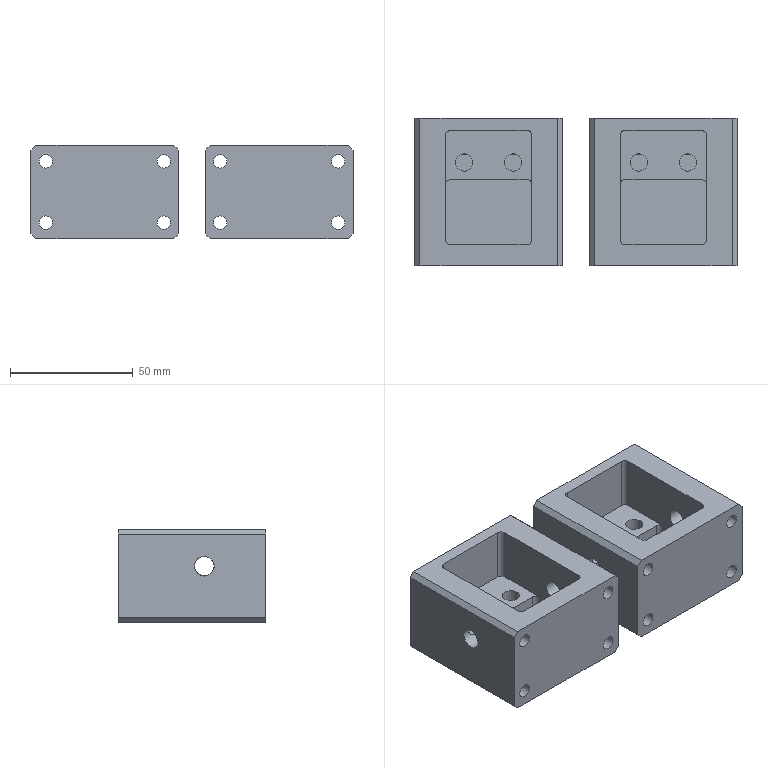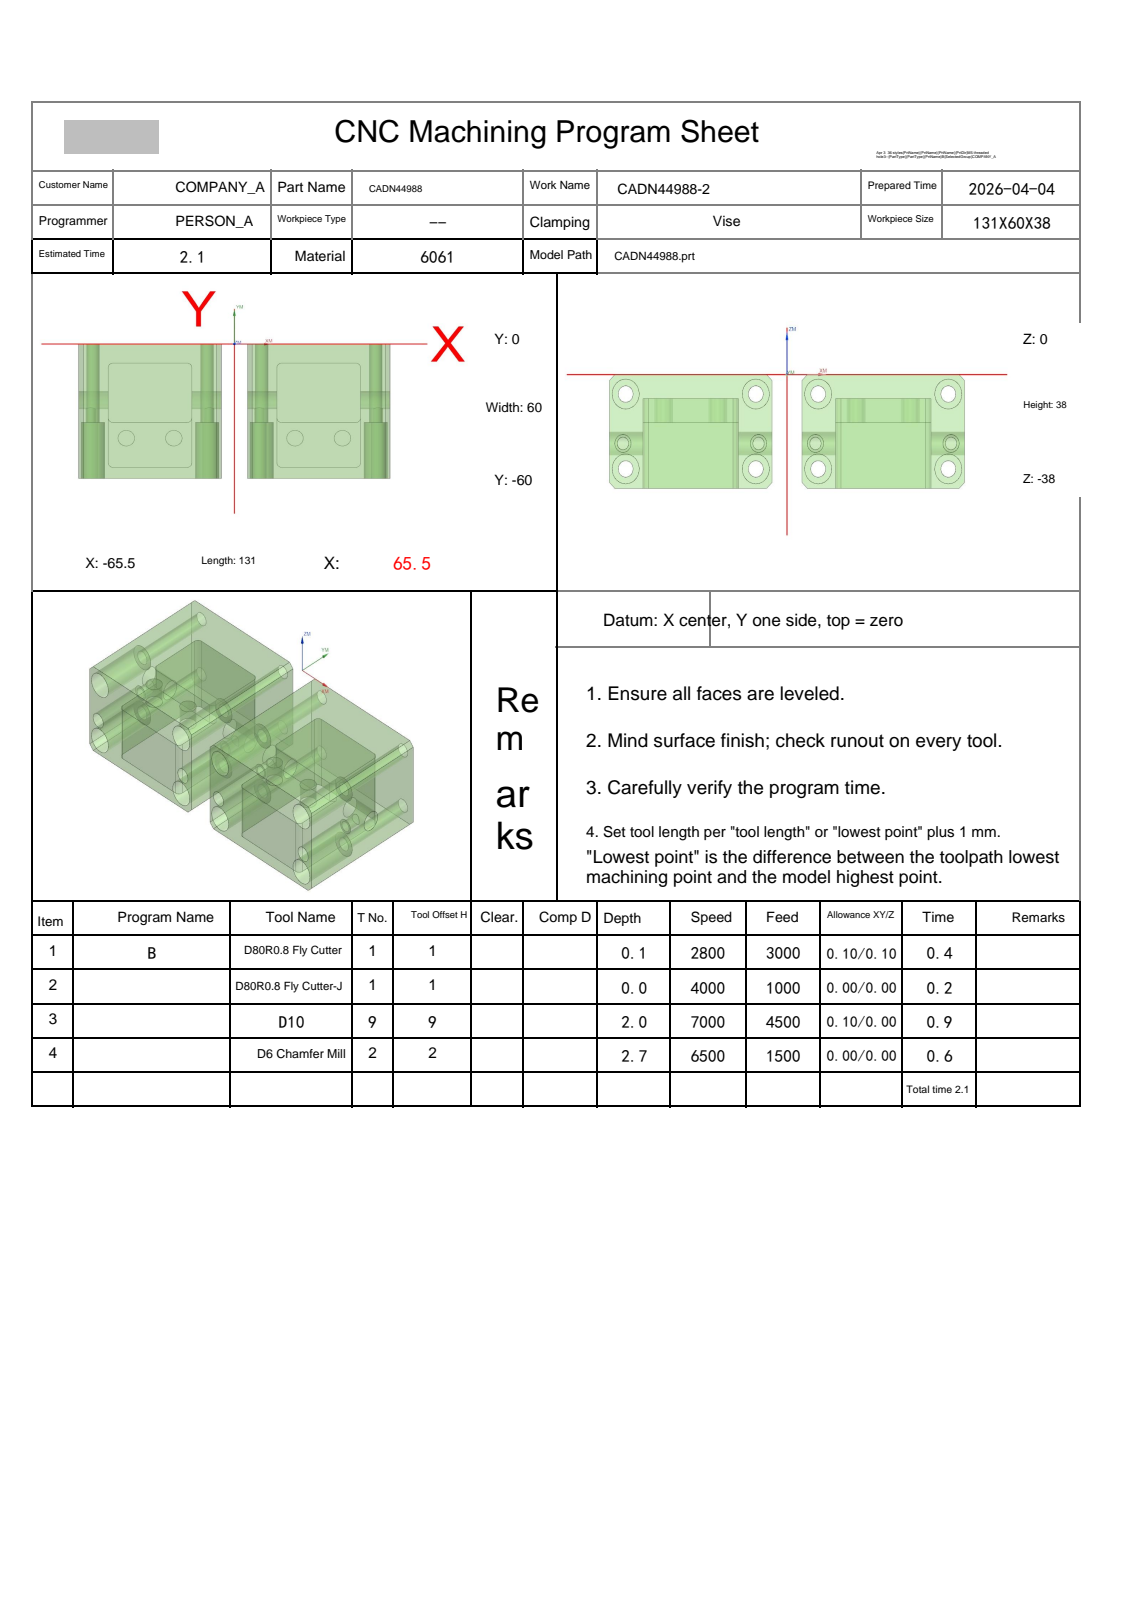NC program | NX | posted by the shop | part box 131 x 60 x 38 mm
Whole program:
%
O0001
(Machine time: 2.90 MIN)
(===Total Tool:3===)
(T1=D80R0.8 Fly Cutter D=80.  R=0.8  D-  H01 Z=0.    )
(T9=D10     D=10.  R=0.   D-  H09 Z=-2.   )
(T2=D6 Chamfer Mill   D=6.   R=0.   D-  H02 Z=-2.7  )
G80 G90 G17 G49 G40
G91 G28 Z0
M01
N1 T01 M06
(D80R0.8 Fly Cutter  D=80. R=0.8 H=01 ce=0.10 di=0.10)
G00 G90 G54 X117.597 Y-30. M03 S2800
G43 H01 Z50.
M08
Z3.525
G01 Z1.525 F3000.
X105.597
X-105.597
X-117.597
Z3.525
G00 X117.597
Z3.05
G01 Z1.05
X105.597
X-105.597
X-117.597
Z3.05
G00 X117.597
Z2.575
G01 Z.575
X105.597
X-105.597
X-117.597
Z2.575
G00 X117.597
Z2.1
G01 Z.1
X105.597
X-105.597
X-117.597
Z2.1
G00 Z50.
G91 G28 Z0.0
M05
M09
G91 G28 Z0.0
M01
N2 T01 M06
(D80R0.8 Fly Cutter-J  D=80. R=0.8 H=01 ce=0.00 di=0.00)
G00 G90 G54 X117.499 Y-30. M03 S4000
G43 H01 Z50.
M08
Z2.
G01 Z0.0 F1000.
X105.499
X-105.499
X-117.499
Z2.
G00 Z50.
G91 G28 Z0.0
M05
M09
G91 G28 Z0.0
M01
N3 T09 M06
(D10  D=10. R=0. H=09 ce=0.10 di=0.00)
G00 G90 G54 X68.442 Y9.956 M03 S7000
G43 H09 Z11.8
M08
Z.359
G01 Z-.141 F4500.
X68.739 Y1.072
X68.741 Y1.014
Y-61.014
X68.739 Y-61.072
X68.812 Z-.212
X68.881 Z-.283
X68.883 Y-61.014
Y1.014
X68.881 Y1.072
X68.954 Z-.354
X69.022 Z-.424
X69.024 Y1.014
Y-61.014
X69.022 Y-61.072
X69.095 Z-.495
X69.164 Z-.566
X69.166 Y-61.014
Y1.014
X69.164 Y1.073
X69.236 Z-.636
X69.305 Z-.707
X69.307 Y1.014
Y-61.014
X69.305 Y-61.073
X69.378 Z-.778
X69.447 Z-.849
X69.449 Y-61.014
Y1.014
X69.447 Y1.073
X69.519 Z-.919
X69.588 Z-.99
X69.59 Y1.014
Y-61.014
X69.588 Y-61.073
X69.661 Z-1.061
X69.729 Z-1.131
X69.731 Y-61.014
Y1.014
X69.729 Y1.073
X69.802 Z-1.202
X69.871 Z-1.273
X69.873 Y1.014
Y-61.014
X69.871 Y-61.073
X69.944 Z-1.344
X70.012 Z-1.414
X70.014 Y-61.014
Y1.014
X70.012 Y1.073
X70.085 Y1.072 Z-1.485
X70.154 Z-1.556
X70.156 Y1.014
Y-61.014
X70.154 Y-61.072
X70.211 Z-1.611
X70.265 Z-1.667
X70.267 Y-61.014
Y1.014
X70.265 Y1.072
X70.322 Z-1.722
X70.376 Z-1.778
X70.378 Y1.014
Y-61.014
X70.376 Y-61.072
X70.433 Z-1.833
X70.487 Z-1.889
X70.489 Y-61.014
Y1.014
X70.487 Y1.072
X70.544 Z-1.944
X70.598 Z-2.
Y-61.072
G00 Z11.8
X2.558 Y-69.955
Z.359
G01 Z-.141
X2.261 Y-61.072
X2.259 Y-61.014
Y1.014
X2.261 Y1.072
X2.188 Z-.212
X2.119 Z-.283
X2.117 Y1.014
Y-61.014
X2.119 Y-61.072
X2.046 Z-.354
X1.978 Z-.424
X1.976 Y-61.014
Y1.014
X1.978 Y1.072
X1.905 Y1.073 Z-.495
X1.836 Z-.566
X1.834 Y1.014
Y-61.014
X1.836 Y-61.073
X1.764 Z-.636
X1.695 Z-.707
X1.693 Y-61.014
Y1.014
X1.695 Y1.073
X1.622 Z-.778
X1.553 Z-.849
X1.551 Y1.014
Y-61.014
X1.553 Y-61.073
X1.481 Z-.919
X1.412 Z-.99
X1.41 Y-61.014
Y1.014
X1.412 Y1.073
X1.339 Z-1.061
X1.271 Z-1.131
X1.269 Y1.014
Y-61.014
X1.271 Y-61.073
X1.198 Z-1.202
X1.129 Z-1.273
X1.127 Y-61.014
Y1.014
X1.129 Y1.073
X1.056 Z-1.344
X.988 Z-1.414
X.986 Y1.014
Y-61.014
X.988 Y-61.073
X.915 Z-1.485
X.846 Y-61.072 Z-1.556
X.844 Y-61.014
Y1.014
X.846 Y1.072
X.789 Z-1.611
X.735 Z-1.667
X.733 Y1.014
Y-61.014
X.735 Y-61.072
X.678 Z-1.722
X.624 Z-1.778
X.622 Y-61.014
Y1.014
X.624 Y1.072
X.567 Z-1.833
X.513 Z-1.889
X.511 Y1.014
Y-61.014
X.513 Y-61.072
X.456 Z-1.944
X.402 Z-2.
Y1.072
G00 Z11.8
X-2.558 Y9.955
Z.359
G01 Z-.141
X-2.261 Y1.072
X-2.259 Y1.014
Y-61.014
X-2.261 Y-61.072
X-2.188 Z-.212
X-2.119 Z-.283
X-2.117 Y-61.014
Y1.014
X-2.119 Y1.072
X-2.046 Z-.354
X-1.978 Z-.424
X-1.976 Y1.014
Y-61.014
X-1.978 Y-61.072
X-1.905 Z-.495
X-1.836 Y-61.073 Z-.566
X-1.834 Y-61.014
Y1.014
X-1.836 Y1.073
X-1.764 Z-.636
X-1.695 Z-.707
X-1.693 Y1.014
Y-61.014
X-1.695 Y-61.073
X-1.622 Z-.778
X-1.553 Z-.849
X-1.551 Y-61.014
Y1.014
X-1.553 Y1.073
X-1.481 Z-.919
X-1.412 Z-.99
X-1.41 Y1.014
Y-61.014
X-1.412 Y-61.073
X-1.339 Z-1.061
X-1.271 Z-1.131
X-1.269 Y-61.014
Y1.014
X-1.271 Y1.073
X-1.198 Z-1.202
X-1.129 Z-1.273
X-1.127 Y1.014
Y-61.014
X-1.129 Y-61.073
X-1.056 Z-1.344
X-.988 Z-1.414
X-.986 Y-61.014
Y1.014
X-.988 Y1.073
X-.915 Y1.072 Z-1.485
X-.846 Z-1.556
X-.844 Y1.014
Y-61.014
X-.846 Y-61.072
X-.789 Z-1.611
X-.735 Z-1.667
X-.733 Y-61.014
Y1.014
X-.735 Y1.072
X-.678 Z-1.722
X-.624 Z-1.778
X-.622 Y1.014
Y-61.014
X-.624 Y-61.072
X-.567 Z-1.833
X-.513 Z-1.889
X-.511 Y-61.014
Y1.014
X-.513 Y1.072
X-.456 Z-1.944
X-.402 Z-2.
Y-61.072
G00 Z11.8
X-68.442 Y-69.956
Z.359
G01 Z-.141
X-68.739 Y-61.072
X-68.741 Y-61.014
Y1.014
X-68.739 Y1.072
X-68.812 Z-.212
X-68.881 Z-.283
X-68.883 Y1.014
Y-61.014
X-68.881 Y-61.072
X-68.954 Z-.354
X-69.022 Z-.424
X-69.024 Y-61.014
Y1.014
X-69.022 Y1.072
X-69.095 Z-.495
X-69.164 Y1.073 Z-.566
X-69.166 Y1.014
Y-61.014
X-69.164 Y-61.072
X-69.236 Y-61.073 Z-.636
X-69.305 Z-.707
X-69.307 Y-61.014
Y1.014
X-69.305 Y1.073
X-69.378 Z-.778
X-69.447 Z-.849
X-69.449 Y1.014
Y-61.014
X-69.447 Y-61.073
X-69.519 Z-.919
X-69.588 Z-.99
X-69.59 Y-61.014
Y1.014
X-69.588 Y1.073
X-69.661 Z-1.061
X-69.729 Z-1.131
X-69.731 Y1.014
Y-61.014
X-69.729 Y-61.073
X-69.802 Z-1.202
X-69.871 Z-1.273
X-69.873 Y-61.014
Y1.014
X-69.871 Y1.073
X-69.944 Z-1.344
X-70.012 Z-1.414
X-70.014 Y1.014
Y-61.014
X-70.012 Y-61.073
X-70.085 Z-1.485
X-70.154 Y-61.072 Z-1.556
X-70.156 Y-61.014
Y1.014
X-70.154 Y1.072
X-70.211 Z-1.611
X-70.265 Z-1.667
X-70.267 Y1.014
Y-61.014
X-70.265 Y-61.072
X-70.322 Z-1.722
X-70.376 Z-1.778
X-70.378 Y-61.014
Y1.014
X-70.376 Y1.072
X-70.433 Z-1.833
X-70.487 Z-1.889
X-70.489 Y1.014
Y-61.014
X-70.487 Y-61.072
X-70.544 Z-1.944
X-70.598 Z-2.
Y1.072
G00 Z11.8
G91 G28 Z0.0
M05
M09
G91 G28 Z0.0
M01
N4 T02 M06
(D6 Chamfer Mill  D=6. R=0. H=02 ce=0.00 di=0.00)
G00 G90 G54 X64.292 Y-60.99 M03 S6500
G43 H02 Z50.
M08
Z.13
G01 Z-1.2 F1500.
G03 X63.952 Y-60.915 I-.601 J-1.907
G01 X63.898 Y-60.905
X63.849 Y-60.928
X63.759 Y-60.966
X63.5 Y-61.
X7.5
X7.241 Y-60.966
X7.151 Y-60.928
X7.102 Y-60.905
X7.048 Y-60.915
G03 X6.708 Y-60.99 I.261 J-1.983
G01 Z.13
G00 Z10.
Y.99
Z.13
G01 Z-1.2
G03 X7.048 Y.915 I.601 J1.907
G01 X7.102 Y.905
X7.151 Y.928
X7.241 Y.966
X7.5 Y1.
X63.5
X63.759 Y.966
X63.849 Y.928
X63.898 Y.905
X63.952 Y.915
G03 X64.292 Y.99 I-.261 J1.983
G01 Z.13
G00 Z10.
X-64.292
Z.13
G01 Z-1.2
G03 X-63.952 Y.915 I.601 J1.907
G01 X-63.898 Y.905
X-63.849 Y.928
X-63.759 Y.966
X-63.5 Y1.
X-7.5
X-7.241 Y.966
X-7.151 Y.928
X-7.102 Y.905
X-7.048 Y.915
G03 X-6.708 Y.99 I-.261 J1.983
G01 Z.13
G00 Z10.
Y-60.99
Z.13
G01 Z-1.2
G03 X-7.048 Y-60.915 I-.601 J-1.907
G01 X-7.102 Y-60.905
X-7.151 Y-60.928
X-7.241 Y-60.966
X-7.5 Y-61.
X-63.5
X-63.759 Y-60.966
X-63.849 Y-60.928
X-63.898 Y-60.905
X-63.952 Y-60.915
G03 X-64.292 Y-60.99 I.261 J-1.983
G01 Z.13
G00 Z50.
G00 G90 X-67.016 Y-63.9 M03 S6500
Z50.
Z-1.2
G01 Z-2.7 F800.
G03 X-66.2 Y-62.763 I-.384 J1.137
G01 Y2.763
G03 X-67.016 Y3.9 I-1.2 J0.0
G01 Z-1.2
G00 Z50.
X-3.984
Z-1.2
G01 Z-2.7
G03 X-4.8 Y2.763 I.384 J-1.137
G01 Y-62.763
G03 X-3.984 Y-63.9 I1.2 J0.0
G01 Z-1.2
G00 X3.984
G01 Z-2.7
G03 X4.8 Y-62.763 I-.384 J1.137
G01 Y2.763
G03 X3.984 Y3.9 I-1.2 J0.0
G01 Z-1.2
G00 Z50.
X67.016
Z-1.2
G01 Z-2.7
G03 X66.2 Y2.763 I.384 J-1.137
G01 Y-62.763
G03 X67.016 Y-63.9 I1.2 J0.0
G01 Z-1.2
G00 Z50.
M05
M09
G91 G28 Z0.0
G91 G28 Y0.0
M30
%